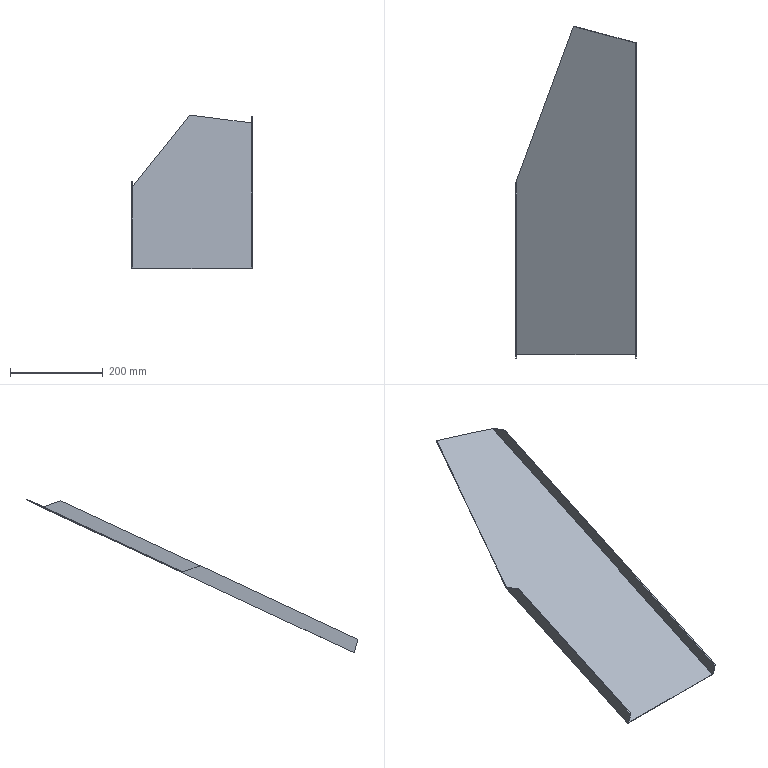Part | NX | features solid 2 | 1 solid | 13 faces | box 260.073 x 716.233 x 332.121 mm | volume 417185 mm3 | plane 13
STEP:
#1=CARTESIAN_POINT('',(826.514,-714.877,-537.036));
#2=VERTEX_POINT('',#1);
#3=CARTESIAN_POINT('',(570.441,-714.877,-537.036));
#4=VERTEX_POINT('',#3);
#5=CARTESIAN_POINT('',(703.453,-714.877,-537.036));
#6=DIRECTION('',(-1.,0.,0.));
#7=VECTOR('',#6,1000.);
#8=LINE('',#5,#7);
#9=EDGE_CURVE('',#2,#4,#8,.T.);
#10=ORIENTED_EDGE('',*,*,#9,.F.);
#11=CARTESIAN_POINT('',(826.514,-43.168,-223.813));
#12=VERTEX_POINT('',#11);
#13=CARTESIAN_POINT('',(826.514,-9.658,-208.187));
#14=DIRECTION('',(0.,-0.9063,-0.4226));
#15=VECTOR('',#14,1000.);
#16=LINE('',#13,#15);
#17=EDGE_CURVE('',#12,#2,#16,.T.);
#18=ORIENTED_EDGE('',*,*,#17,.F.);
#19=CARTESIAN_POINT('',(828.514,-43.168,-223.813));
#20=VERTEX_POINT('',#19);
#21=CARTESIAN_POINT('',(828.514,-43.168,-223.813));
#22=DIRECTION('',(1.,0.,0.));
#23=VECTOR('',#22,1000.);
#24=LINE('',#21,#23);
#25=EDGE_CURVE('',#12,#20,#24,.T.);
#26=ORIENTED_EDGE('',*,*,#25,.T.);
#27=CARTESIAN_POINT('',(692.963,-6.847,-206.877));
#28=VERTEX_POINT('',#27);
#29=CARTESIAN_POINT('',(703.453,-9.658,-208.187));
#30=DIRECTION('',(-0.959,0.257,0.1198));
#31=VECTOR('',#30,1000.);
#32=LINE('',#29,#31);
#33=EDGE_CURVE('',#20,#28,#32,.T.);
#34=ORIENTED_EDGE('',*,*,#33,.T.);
#35=CARTESIAN_POINT('',(568.441,-344.388,-364.275));
#36=VERTEX_POINT('',#35);
#37=CARTESIAN_POINT('',(693.085,-6.517,-206.722));
#38=DIRECTION('',(0.3171,0.8595,0.4008));
#39=VECTOR('',#38,1000.);
#40=LINE('',#37,#39);
#41=EDGE_CURVE('',#36,#28,#40,.T.);
#42=ORIENTED_EDGE('',*,*,#41,.F.);
#43=CARTESIAN_POINT('',(570.441,-344.388,-364.275));
#44=VERTEX_POINT('',#43);
#45=CARTESIAN_POINT('',(568.441,-344.388,-364.275));
#46=DIRECTION('',(-1.,0.,0.));
#47=VECTOR('',#46,1000.);
#48=LINE('',#45,#47);
#49=EDGE_CURVE('',#36,#44,#48,.F.);
#50=ORIENTED_EDGE('',*,*,#49,.T.);
#51=CARTESIAN_POINT('',(570.441,-9.658,-208.187));
#52=DIRECTION('',(0.,-0.9063,-0.4226));
#53=VECTOR('',#52,1000.);
#54=LINE('',#51,#53);
#55=EDGE_CURVE('',#44,#4,#54,.T.);
#56=ORIENTED_EDGE('',*,*,#55,.T.);
#57=EDGE_LOOP('',(#10,#18,#26,#34,#42,#50,#56));
#58=FACE_BOUND('',#57,.T.);
#59=CARTESIAN_POINT('',(703.453,-9.658,-208.187));
#60=DIRECTION('',(0.,-0.4226,0.9063));
#61=DIRECTION('',(1.,0.,0.));
#62=AXIS2_PLACEMENT_3D('',#59,#60,#61);
#63=PLANE('',#62);
#64=ADVANCED_FACE('',(#58),#63,.T.);
#65=CARTESIAN_POINT('',(828.514,-714.351,-538.998));
#66=VERTEX_POINT('',#65);
#67=CARTESIAN_POINT('',(828.514,-722.236,-509.573));
#68=VERTEX_POINT('',#67);
#69=CARTESIAN_POINT('',(828.514,-749.848,-406.521));
#70=DIRECTION('',(0.,-0.2588,0.9659));
#71=VECTOR('',#70,1000.);
#72=LINE('',#69,#71);
#73=EDGE_CURVE('',#66,#68,#72,.T.);
#74=ORIENTED_EDGE('',*,*,#73,.F.);
#75=CARTESIAN_POINT('',(828.514,-42.323,-225.626));
#76=VERTEX_POINT('',#75);
#77=CARTESIAN_POINT('',(828.514,-8.813,-210.));
#78=DIRECTION('',(0.,-0.9063,-0.4226));
#79=VECTOR('',#78,1000.);
#80=LINE('',#77,#79);
#81=EDGE_CURVE('',#76,#66,#80,.T.);
#82=ORIENTED_EDGE('',*,*,#81,.F.);
#83=CARTESIAN_POINT('',(828.514,-43.168,-223.813));
#84=DIRECTION('',(0.,0.4226,-0.9063));
#85=VECTOR('',#84,1000.);
#86=LINE('',#83,#85);
#87=EDGE_CURVE('',#20,#76,#86,.T.);
#88=ORIENTED_EDGE('',*,*,#87,.F.);
#89=CARTESIAN_POINT('',(828.514,-80.378,-210.27));
#90=VERTEX_POINT('',#89);
#91=CARTESIAN_POINT('',(828.514,-80.378,-210.27));
#92=DIRECTION('',(0.,0.9397,-0.342));
#93=VECTOR('',#92,1000.);
#94=LINE('',#91,#93);
#95=EDGE_CURVE('',#20,#90,#94,.F.);
#96=ORIENTED_EDGE('',*,*,#95,.T.);
#97=CARTESIAN_POINT('',(828.514,-55.002,-198.437));
#98=DIRECTION('',(0.,-0.9063,-0.4226));
#99=VECTOR('',#98,1000.);
#100=LINE('',#97,#99);
#101=EDGE_CURVE('',#90,#68,#100,.T.);
#102=ORIENTED_EDGE('',*,*,#101,.T.);
#103=EDGE_LOOP('',(#74,#82,#88,#96,#102));
#104=FACE_BOUND('',#103,.T.);
#105=CARTESIAN_POINT('',(828.514,-9.658,-208.187));
#106=DIRECTION('',(1.,0.,0.));
#107=DIRECTION('',(0.,1.,0.));
#108=AXIS2_PLACEMENT_3D('',#105,#106,#107);
#109=PLANE('',#108);
#110=ADVANCED_FACE('',(#104),#109,.T.);
#111=CARTESIAN_POINT('',(692.963,-6.002,-208.689));
#112=VERTEX_POINT('',#111);
#113=CARTESIAN_POINT('',(703.453,-8.813,-210.));
#114=DIRECTION('',(-0.959,0.257,0.1198));
#115=VECTOR('',#114,1000.);
#116=LINE('',#113,#115);
#117=EDGE_CURVE('',#76,#112,#116,.T.);
#118=ORIENTED_EDGE('',*,*,#117,.T.);
#119=CARTESIAN_POINT('',(692.963,-6.847,-206.877));
#120=DIRECTION('',(0.,0.4226,-0.9063));
#121=VECTOR('',#120,1000.);
#122=LINE('',#119,#121);
#123=EDGE_CURVE('',#28,#112,#122,.T.);
#124=ORIENTED_EDGE('',*,*,#123,.F.);
#125=ORIENTED_EDGE('',*,*,#33,.F.);
#126=ORIENTED_EDGE('',*,*,#87,.T.);
#127=EDGE_LOOP('',(#118,#124,#125,#126));
#128=FACE_BOUND('',#127,.T.);
#129=CARTESIAN_POINT('',(703.453,-9.658,-208.187));
#130=DIRECTION('',(-0.2835,-0.8691,-0.4053));
#131=DIRECTION('',(0.,0.4226,-0.9063));
#132=AXIS2_PLACEMENT_3D('',#129,#130,#131);
#133=PLANE('',#132);
#134=ADVANCED_FACE('',(#128),#133,.F.);
#135=CARTESIAN_POINT('',(568.441,-343.543,-366.087));
#136=VERTEX_POINT('',#135);
#137=CARTESIAN_POINT('',(693.085,-5.671,-208.535));
#138=DIRECTION('',(0.3171,0.8595,0.4008));
#139=VECTOR('',#138,1000.);
#140=LINE('',#137,#139);
#141=EDGE_CURVE('',#136,#112,#140,.T.);
#142=ORIENTED_EDGE('',*,*,#141,.F.);
#143=CARTESIAN_POINT('',(568.441,-344.388,-364.275));
#144=DIRECTION('',(0.,0.4226,-0.9063));
#145=VECTOR('',#144,1000.);
#146=LINE('',#143,#145);
#147=EDGE_CURVE('',#36,#136,#146,.T.);
#148=ORIENTED_EDGE('',*,*,#147,.F.);
#149=ORIENTED_EDGE('',*,*,#41,.T.);
#150=ORIENTED_EDGE('',*,*,#123,.T.);
#151=EDGE_LOOP('',(#142,#148,#149,#150));
#152=FACE_BOUND('',#151,.T.);
#153=CARTESIAN_POINT('',(693.085,-6.517,-206.722));
#154=DIRECTION('',(-0.9484,0.2874,0.134));
#155=DIRECTION('',(-0.29,-0.957,0.));
#156=AXIS2_PLACEMENT_3D('',#153,#154,#155);
#157=PLANE('',#156);
#158=ADVANCED_FACE('',(#152),#157,.T.);
#159=CARTESIAN_POINT('',(568.441,-714.351,-538.998));
#160=VERTEX_POINT('',#159);
#161=CARTESIAN_POINT('',(568.441,-8.813,-210.));
#162=DIRECTION('',(0.,-0.9063,-0.4226));
#163=VECTOR('',#162,1000.);
#164=LINE('',#161,#163);
#165=EDGE_CURVE('',#136,#160,#164,.T.);
#166=ORIENTED_EDGE('',*,*,#165,.T.);
#167=CARTESIAN_POINT('',(568.441,-722.236,-509.573));
#168=VERTEX_POINT('',#167);
#169=CARTESIAN_POINT('',(568.441,-749.848,-406.521));
#170=DIRECTION('',(0.,-0.2588,0.9659));
#171=VECTOR('',#170,1000.);
#172=LINE('',#169,#171);
#173=EDGE_CURVE('',#160,#168,#172,.T.);
#174=ORIENTED_EDGE('',*,*,#173,.T.);
#175=CARTESIAN_POINT('',(568.441,-381.598,-350.731));
#176=VERTEX_POINT('',#175);
#177=CARTESIAN_POINT('',(568.441,-356.222,-338.898));
#178=DIRECTION('',(0.,-0.9063,-0.4226));
#179=VECTOR('',#178,1000.);
#180=LINE('',#177,#179);
#181=EDGE_CURVE('',#176,#168,#180,.T.);
#182=ORIENTED_EDGE('',*,*,#181,.F.);
#183=CARTESIAN_POINT('',(568.441,-343.06,-364.758));
#184=DIRECTION('',(0.,-0.9397,0.342));
#185=VECTOR('',#184,1000.);
#186=LINE('',#183,#185);
#187=EDGE_CURVE('',#176,#36,#186,.F.);
#188=ORIENTED_EDGE('',*,*,#187,.T.);
#189=ORIENTED_EDGE('',*,*,#147,.T.);
#190=EDGE_LOOP('',(#166,#174,#182,#188,#189));
#191=FACE_BOUND('',#190,.T.);
#192=CARTESIAN_POINT('',(568.441,-9.658,-208.187));
#193=DIRECTION('',(1.,0.,0.));
#194=DIRECTION('',(0.,1.,0.));
#195=AXIS2_PLACEMENT_3D('',#192,#193,#194);
#196=PLANE('',#195);
#197=ADVANCED_FACE('',(#191),#196,.F.);
#198=ORIENTED_EDGE('',*,*,#81,.T.);
#199=CARTESIAN_POINT('',(703.453,-714.351,-538.998));
#200=DIRECTION('',(-1.,0.,0.));
#201=VECTOR('',#200,1000.);
#202=LINE('',#199,#201);
#203=EDGE_CURVE('',#66,#160,#202,.T.);
#204=ORIENTED_EDGE('',*,*,#203,.T.);
#205=ORIENTED_EDGE('',*,*,#165,.F.);
#206=ORIENTED_EDGE('',*,*,#141,.T.);
#207=ORIENTED_EDGE('',*,*,#117,.F.);
#208=EDGE_LOOP('',(#198,#204,#205,#206,#207));
#209=FACE_BOUND('',#208,.T.);
#210=CARTESIAN_POINT('',(703.453,-8.813,-210.));
#211=DIRECTION('',(0.,-0.4226,0.9063));
#212=DIRECTION('',(1.,0.,0.));
#213=AXIS2_PLACEMENT_3D('',#210,#211,#212);
#214=PLANE('',#213);
#215=ADVANCED_FACE('',(#209),#214,.F.);
#216=CARTESIAN_POINT('',(570.441,-722.236,-509.573));
#217=VERTEX_POINT('',#216);
#218=CARTESIAN_POINT('',(568.441,-722.236,-509.573));
#219=DIRECTION('',(1.,0.,0.));
#220=VECTOR('',#219,1000.);
#221=LINE('',#218,#220);
#222=EDGE_CURVE('',#217,#168,#221,.F.);
#223=ORIENTED_EDGE('',*,*,#222,.F.);
#224=CARTESIAN_POINT('',(570.441,-381.598,-350.731));
#225=VERTEX_POINT('',#224);
#226=CARTESIAN_POINT('',(570.441,-356.222,-338.898));
#227=DIRECTION('',(0.,-0.9063,-0.4226));
#228=VECTOR('',#227,1000.);
#229=LINE('',#226,#228);
#230=EDGE_CURVE('',#225,#217,#229,.T.);
#231=ORIENTED_EDGE('',*,*,#230,.F.);
#232=CARTESIAN_POINT('',(568.441,-381.598,-350.731));
#233=DIRECTION('',(1.,0.,0.));
#234=VECTOR('',#233,1000.);
#235=LINE('',#232,#234);
#236=EDGE_CURVE('',#225,#176,#235,.F.);
#237=ORIENTED_EDGE('',*,*,#236,.T.);
#238=ORIENTED_EDGE('',*,*,#181,.T.);
#239=EDGE_LOOP('',(#223,#231,#237,#238));
#240=FACE_BOUND('',#239,.T.);
#241=CARTESIAN_POINT('',(568.441,-356.222,-338.898));
#242=DIRECTION('',(0.,0.4226,-0.9063));
#243=DIRECTION('',(0.,-0.9063,-0.4226));
#244=AXIS2_PLACEMENT_3D('',#241,#242,#243);
#245=PLANE('',#244);
#246=ADVANCED_FACE('',(#240),#245,.F.);
#247=ORIENTED_EDGE('',*,*,#230,.T.);
#248=CARTESIAN_POINT('',(570.441,-732.74,-470.372));
#249=DIRECTION('',(0.,0.2588,-0.9659));
#250=VECTOR('',#249,1000.);
#251=LINE('',#248,#250);
#252=EDGE_CURVE('',#217,#4,#251,.T.);
#253=ORIENTED_EDGE('',*,*,#252,.T.);
#254=ORIENTED_EDGE('',*,*,#55,.F.);
#255=CARTESIAN_POINT('',(570.441,-344.388,-364.275));
#256=DIRECTION('',(0.,0.9397,-0.342));
#257=VECTOR('',#256,1000.);
#258=LINE('',#255,#257);
#259=EDGE_CURVE('',#44,#225,#258,.F.);
#260=ORIENTED_EDGE('',*,*,#259,.T.);
#261=EDGE_LOOP('',(#247,#253,#254,#260));
#262=FACE_BOUND('',#261,.T.);
#263=CARTESIAN_POINT('',(570.441,-343.543,-366.087));
#264=DIRECTION('',(-1.,0.,0.));
#265=DIRECTION('',(0.,-1.,0.));
#266=AXIS2_PLACEMENT_3D('',#263,#264,#265);
#267=PLANE('',#266);
#268=ADVANCED_FACE('',(#262),#267,.F.);
#269=ORIENTED_EDGE('',*,*,#187,.F.);
#270=ORIENTED_EDGE('',*,*,#236,.F.);
#271=ORIENTED_EDGE('',*,*,#259,.F.);
#272=ORIENTED_EDGE('',*,*,#49,.F.);
#273=EDGE_LOOP('',(#269,#270,#271,#272));
#274=FACE_BOUND('',#273,.T.);
#275=CARTESIAN_POINT('',(568.441,-344.388,-364.275));
#276=DIRECTION('',(0.,-0.342,-0.9397));
#277=DIRECTION('',(0.,0.9397,-0.342));
#278=AXIS2_PLACEMENT_3D('',#275,#276,#277);
#279=PLANE('',#278);
#280=ADVANCED_FACE('',(#274),#279,.F.);
#281=CARTESIAN_POINT('',(826.514,-80.378,-210.27));
#282=VERTEX_POINT('',#281);
#283=CARTESIAN_POINT('',(826.514,-722.236,-509.573));
#284=VERTEX_POINT('',#283);
#285=CARTESIAN_POINT('',(826.514,-55.002,-198.437));
#286=DIRECTION('',(0.,-0.9063,-0.4226));
#287=VECTOR('',#286,1000.);
#288=LINE('',#285,#287);
#289=EDGE_CURVE('',#282,#284,#288,.T.);
#290=ORIENTED_EDGE('',*,*,#289,.T.);
#291=CARTESIAN_POINT('',(828.514,-722.236,-509.573));
#292=DIRECTION('',(1.,0.,0.));
#293=VECTOR('',#292,1000.);
#294=LINE('',#291,#293);
#295=EDGE_CURVE('',#284,#68,#294,.T.);
#296=ORIENTED_EDGE('',*,*,#295,.T.);
#297=ORIENTED_EDGE('',*,*,#101,.F.);
#298=CARTESIAN_POINT('',(828.514,-80.378,-210.27));
#299=DIRECTION('',(-1.,0.,0.));
#300=VECTOR('',#299,1000.);
#301=LINE('',#298,#300);
#302=EDGE_CURVE('',#90,#282,#301,.T.);
#303=ORIENTED_EDGE('',*,*,#302,.T.);
#304=EDGE_LOOP('',(#290,#296,#297,#303));
#305=FACE_BOUND('',#304,.T.);
#306=CARTESIAN_POINT('',(828.514,-55.002,-198.437));
#307=DIRECTION('',(0.,0.4226,-0.9063));
#308=DIRECTION('',(0.,-0.9063,-0.4226));
#309=AXIS2_PLACEMENT_3D('',#306,#307,#308);
#310=PLANE('',#309);
#311=ADVANCED_FACE('',(#305),#310,.F.);
#312=CARTESIAN_POINT('',(826.514,-747.677,-414.625));
#313=DIRECTION('',(0.,0.2588,-0.9659));
#314=VECTOR('',#313,1000.);
#315=LINE('',#312,#314);
#316=EDGE_CURVE('',#284,#2,#315,.T.);
#317=ORIENTED_EDGE('',*,*,#316,.F.);
#318=ORIENTED_EDGE('',*,*,#289,.F.);
#319=CARTESIAN_POINT('',(826.514,-41.839,-224.297));
#320=DIRECTION('',(0.,-0.9397,0.342));
#321=VECTOR('',#320,1000.);
#322=LINE('',#319,#321);
#323=EDGE_CURVE('',#282,#12,#322,.F.);
#324=ORIENTED_EDGE('',*,*,#323,.T.);
#325=ORIENTED_EDGE('',*,*,#17,.T.);
#326=EDGE_LOOP('',(#317,#318,#324,#325));
#327=FACE_BOUND('',#326,.T.);
#328=CARTESIAN_POINT('',(826.514,-42.323,-225.626));
#329=DIRECTION('',(-1.,0.,0.));
#330=DIRECTION('',(0.,-1.,0.));
#331=AXIS2_PLACEMENT_3D('',#328,#329,#330);
#332=PLANE('',#331);
#333=ADVANCED_FACE('',(#327),#332,.T.);
#334=ORIENTED_EDGE('',*,*,#95,.F.);
#335=ORIENTED_EDGE('',*,*,#25,.F.);
#336=ORIENTED_EDGE('',*,*,#323,.F.);
#337=ORIENTED_EDGE('',*,*,#302,.F.);
#338=EDGE_LOOP('',(#334,#335,#336,#337));
#339=FACE_BOUND('',#338,.T.);
#340=CARTESIAN_POINT('',(828.514,-80.378,-210.27));
#341=DIRECTION('',(0.,-0.342,-0.9397));
#342=DIRECTION('',(0.,0.9397,-0.342));
#343=AXIS2_PLACEMENT_3D('',#340,#341,#342);
#344=PLANE('',#343);
#345=ADVANCED_FACE('',(#339),#344,.F.);
#346=ORIENTED_EDGE('',*,*,#173,.F.);
#347=ORIENTED_EDGE('',*,*,#203,.F.);
#348=ORIENTED_EDGE('',*,*,#73,.T.);
#349=ORIENTED_EDGE('',*,*,#295,.F.);
#350=ORIENTED_EDGE('',*,*,#316,.T.);
#351=ORIENTED_EDGE('',*,*,#9,.T.);
#352=ORIENTED_EDGE('',*,*,#252,.F.);
#353=ORIENTED_EDGE('',*,*,#222,.T.);
#354=EDGE_LOOP('',(#346,#347,#348,#349,#350,#351,#352,#353));
#355=FACE_BOUND('',#354,.T.);
#356=CARTESIAN_POINT('',(830.,-710.87,-551.991));
#357=DIRECTION('',(0.,0.9659,0.2588));
#358=DIRECTION('',(0.,-0.2588,0.9659));
#359=AXIS2_PLACEMENT_3D('',#356,#357,#358);
#360=PLANE('',#359);
#361=ADVANCED_FACE('',(#355),#360,.F.);
#362=CLOSED_SHELL('',(#64,#110,#134,#158,#197,#215,#246,#268,#280,#311,#333,#345,#361));
#363=MANIFOLD_SOLID_BREP('',#362);
#364=(LENGTH_UNIT()NAMED_UNIT(*)SI_UNIT(.MILLI.,.METRE.));
#365=UNCERTAINTY_MEASURE_WITH_UNIT(LENGTH_MEASURE(0.00001),#364,'','');
#366=(NAMED_UNIT(*)PLANE_ANGLE_UNIT()SI_UNIT($,.RADIAN.));
#367=(NAMED_UNIT(*)SI_UNIT($,.STERADIAN.)SOLID_ANGLE_UNIT());
#368=(GEOMETRIC_REPRESENTATION_CONTEXT(3)GLOBAL_UNCERTAINTY_ASSIGNED_CONTEXT((#365))GLOBAL_UNIT_ASSIGNED_CONTEXT((#364,#366,#367))REPRESENTATION_CONTEXT('',''));
#369=ADVANCED_BREP_SHAPE_REPRESENTATION('',(#363),#368);